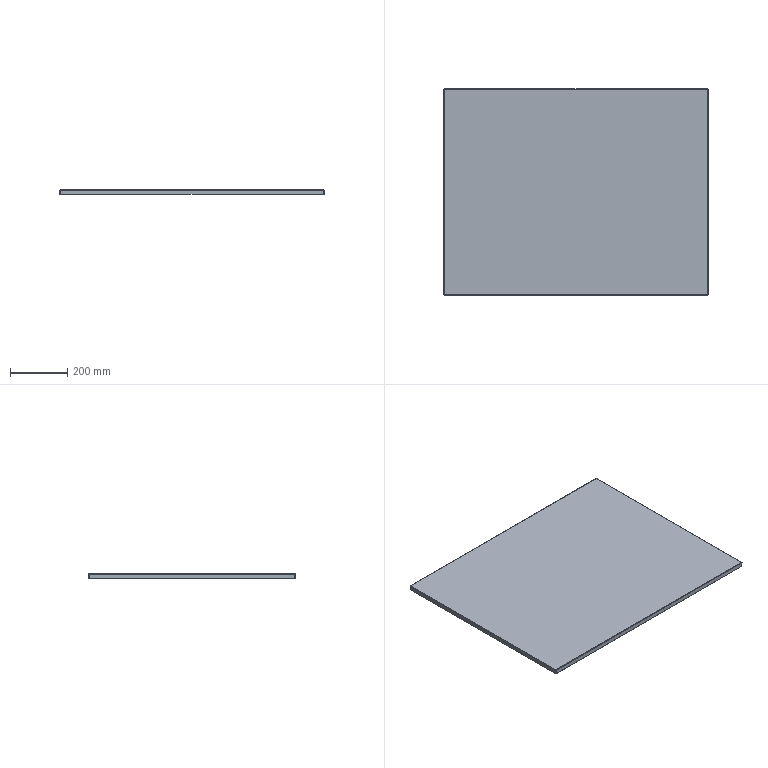Part | STEP file | Base plate | 1 solid | 38 faces | box 919 x 719 x 16.2 mm | volume 850250 mm3 | plane 22 | spline 8 | cylinder 8 | commonest cylinder face diameters 0.4 x4 2.8 x4
STEP:
#1=CARTESIAN_POINT('',(458.1,358.1,-1.2));
#2=VERTEX_POINT('',#1);
#3=CARTESIAN_POINT('',(-458.1,358.1,-1.2));
#4=VERTEX_POINT('',#3);
#5=CARTESIAN_POINT('',(458.1,358.1,-1.2));
#6=DIRECTION('',(-1.,0.,0.));
#7=VECTOR('',#6,1000.);
#8=LINE('',#5,#7);
#9=EDGE_CURVE('',#2,#4,#8,.T.);
#10=ORIENTED_EDGE('',*,*,#9,.F.);
#11=CARTESIAN_POINT('',(458.1,-358.1,-1.2));
#12=VERTEX_POINT('',#11);
#13=CARTESIAN_POINT('',(458.1,-358.1,-1.2));
#14=DIRECTION('',(0.,1.,0.));
#15=VECTOR('',#14,1000.);
#16=LINE('',#13,#15);
#17=EDGE_CURVE('',#12,#2,#16,.T.);
#18=ORIENTED_EDGE('',*,*,#17,.F.);
#19=CARTESIAN_POINT('',(-458.1,-358.1,-1.2));
#20=VERTEX_POINT('',#19);
#21=CARTESIAN_POINT('',(-458.1,-358.1,-1.2));
#22=DIRECTION('',(1.,0.,0.));
#23=VECTOR('',#22,1000.);
#24=LINE('',#21,#23);
#25=EDGE_CURVE('',#20,#12,#24,.T.);
#26=ORIENTED_EDGE('',*,*,#25,.F.);
#27=CARTESIAN_POINT('',(-458.1,358.1,-1.2));
#28=DIRECTION('',(0.,-1.,0.));
#29=VECTOR('',#28,1000.);
#30=LINE('',#27,#29);
#31=EDGE_CURVE('',#4,#20,#30,.T.);
#32=ORIENTED_EDGE('',*,*,#31,.F.);
#33=EDGE_LOOP('',(#10,#18,#26,#32));
#34=FACE_OUTER_BOUND('',#33,.T.);
#35=CARTESIAN_POINT('',(0.,0.,-1.2));
#36=DIRECTION('',(0.,0.,1.));
#37=DIRECTION('',(1.,0.,0.));
#38=AXIS2_PLACEMENT_3D('',#35,#36,#37);
#39=PLANE('',#38);
#40=ADVANCED_FACE('',(#34),#39,.F.);
#41=CARTESIAN_POINT('',(458.1,-358.1,0.));
#42=VERTEX_POINT('',#41);
#43=CARTESIAN_POINT('',(458.1,358.1,0.));
#44=VERTEX_POINT('',#43);
#45=CARTESIAN_POINT('',(458.1,-358.1,0.));
#46=DIRECTION('',(0.,1.,0.));
#47=VECTOR('',#46,1000.);
#48=LINE('',#45,#47);
#49=EDGE_CURVE('',#42,#44,#48,.T.);
#50=ORIENTED_EDGE('',*,*,#49,.T.);
#51=CARTESIAN_POINT('',(-458.1,358.1,0.));
#52=VERTEX_POINT('',#51);
#53=CARTESIAN_POINT('',(458.1,358.1,0.));
#54=DIRECTION('',(-1.,0.,0.));
#55=VECTOR('',#54,1000.);
#56=LINE('',#53,#55);
#57=EDGE_CURVE('',#44,#52,#56,.T.);
#58=ORIENTED_EDGE('',*,*,#57,.T.);
#59=CARTESIAN_POINT('',(-458.1,-358.1,0.));
#60=VERTEX_POINT('',#59);
#61=CARTESIAN_POINT('',(-458.1,358.1,0.));
#62=DIRECTION('',(0.,-1.,0.));
#63=VECTOR('',#62,1000.);
#64=LINE('',#61,#63);
#65=EDGE_CURVE('',#52,#60,#64,.T.);
#66=ORIENTED_EDGE('',*,*,#65,.T.);
#67=CARTESIAN_POINT('',(-458.1,-358.1,0.));
#68=DIRECTION('',(1.,0.,0.));
#69=VECTOR('',#68,1000.);
#70=LINE('',#67,#69);
#71=EDGE_CURVE('',#60,#42,#70,.T.);
#72=ORIENTED_EDGE('',*,*,#71,.T.);
#73=EDGE_LOOP('',(#50,#58,#66,#72));
#74=FACE_OUTER_BOUND('',#73,.T.);
#75=CARTESIAN_POINT('',(0.,0.,0.));
#76=DIRECTION('',(0.,0.,1.));
#77=DIRECTION('',(1.,0.,0.));
#78=AXIS2_PLACEMENT_3D('',#75,#76,#77);
#79=PLANE('',#78);
#80=ADVANCED_FACE('',(#74),#79,.T.);
#81=CARTESIAN_POINT('',(457.593,-359.5,-1.4));
#82=VERTEX_POINT('',#81);
#83=CARTESIAN_POINT('',(457.593,-358.3,-1.4));
#84=VERTEX_POINT('',#83);
#85=CARTESIAN_POINT('',(457.593,-358.3,-1.4));
#86=DIRECTION('',(0.,1.,0.));
#87=VECTOR('',#86,1000.);
#88=LINE('',#85,#87);
#89=EDGE_CURVE('',#82,#84,#88,.T.);
#90=ORIENTED_EDGE('',*,*,#89,.T.);
#91=CARTESIAN_POINT('',(458.1,-358.1,-1.2));
#92=CARTESIAN_POINT('',(458.015,-358.152,-1.2));
#93=CARTESIAN_POINT('',(457.931,-358.204,-1.222));
#94=CARTESIAN_POINT('',(457.762,-358.278,-1.296));
#95=CARTESIAN_POINT('',(457.677,-358.3,-1.348));
#96=CARTESIAN_POINT('',(457.593,-358.3,-1.4));
#97=B_SPLINE_CURVE_WITH_KNOTS('',3,(#91,#92,#93,#94,#95,#96),.UNSPECIFIED.,.F.,.F.,(4,2,4),(0.,0.5,1.),.UNSPECIFIED.);
#98=EDGE_CURVE('',#12,#84,#97,.T.);
#99=ORIENTED_EDGE('',*,*,#98,.F.);
#100=CARTESIAN_POINT('',(458.1,-358.1,-1.2));
#101=DIRECTION('',(0.,0.,1.));
#102=VECTOR('',#101,1000.);
#103=LINE('',#100,#102);
#104=EDGE_CURVE('',#12,#42,#103,.T.);
#105=ORIENTED_EDGE('',*,*,#104,.T.);
#106=CARTESIAN_POINT('',(458.1,-358.1,0.));
#107=CARTESIAN_POINT('',(458.058,-358.283,0.));
#108=CARTESIAN_POINT('',(458.015,-358.466,-0.03644));
#109=CARTESIAN_POINT('',(457.931,-358.805,-0.1767));
#110=CARTESIAN_POINT('',(457.889,-358.96,-0.2805));
#111=CARTESIAN_POINT('',(457.804,-359.22,-0.5396));
#112=CARTESIAN_POINT('',(457.762,-359.323,-0.6949));
#113=CARTESIAN_POINT('',(457.677,-359.464,-1.034));
#114=CARTESIAN_POINT('',(457.635,-359.5,-1.217));
#115=CARTESIAN_POINT('',(457.593,-359.5,-1.4));
#116=B_SPLINE_CURVE_WITH_KNOTS('',3,(#106,#107,#108,#109,#110,#111,#112,#113,#114,#115),.UNSPECIFIED.,.F.,.F.,(4,2,2,2,4),(0.,0.25,0.5,0.75,1.),.UNSPECIFIED.);
#117=EDGE_CURVE('',#42,#82,#116,.T.);
#118=ORIENTED_EDGE('',*,*,#117,.T.);
#119=EDGE_LOOP('',(#90,#99,#105,#118));
#120=FACE_OUTER_BOUND('',#119,.T.);
#121=CARTESIAN_POINT('',(458.1,-358.1,0.012));
#122=CARTESIAN_POINT('',(458.058,-358.285,0.012));
#123=CARTESIAN_POINT('',(458.015,-358.47,-0.02475));
#124=CARTESIAN_POINT('',(457.931,-358.811,-0.1662));
#125=CARTESIAN_POINT('',(457.889,-358.968,-0.2709));
#126=CARTESIAN_POINT('',(457.804,-359.229,-0.5323));
#127=CARTESIAN_POINT('',(457.762,-359.334,-0.6889));
#128=CARTESIAN_POINT('',(457.677,-359.475,-1.03));
#129=CARTESIAN_POINT('',(457.635,-359.512,-1.215));
#130=CARTESIAN_POINT('',(457.593,-359.512,-1.4));
#131=CARTESIAN_POINT('',(458.1,-358.1,0.));
#132=CARTESIAN_POINT('',(458.058,-358.283,0.));
#133=CARTESIAN_POINT('',(458.015,-358.466,-0.03644));
#134=CARTESIAN_POINT('',(457.931,-358.805,-0.1767));
#135=CARTESIAN_POINT('',(457.889,-358.96,-0.2805));
#136=CARTESIAN_POINT('',(457.804,-359.22,-0.5396));
#137=CARTESIAN_POINT('',(457.762,-359.323,-0.6949));
#138=CARTESIAN_POINT('',(457.677,-359.464,-1.034));
#139=CARTESIAN_POINT('',(457.635,-359.5,-1.217));
#140=CARTESIAN_POINT('',(457.593,-359.5,-1.4));
#141=CARTESIAN_POINT('',(458.1,-358.1,-1.2));
#142=CARTESIAN_POINT('',(458.058,-358.126,-1.2));
#143=CARTESIAN_POINT('',(458.015,-358.152,-1.205));
#144=CARTESIAN_POINT('',(457.931,-358.201,-1.225));
#145=CARTESIAN_POINT('',(457.889,-358.223,-1.24));
#146=CARTESIAN_POINT('',(457.804,-358.26,-1.277));
#147=CARTESIAN_POINT('',(457.762,-358.275,-1.299));
#148=CARTESIAN_POINT('',(457.677,-358.295,-1.348));
#149=CARTESIAN_POINT('',(457.635,-358.3,-1.374));
#150=CARTESIAN_POINT('',(457.593,-358.3,-1.4));
#151=CARTESIAN_POINT('',(458.1,-358.1,-1.212));
#152=CARTESIAN_POINT('',(458.058,-358.125,-1.212));
#153=CARTESIAN_POINT('',(458.015,-358.149,-1.217));
#154=CARTESIAN_POINT('',(457.931,-358.195,-1.236));
#155=CARTESIAN_POINT('',(457.889,-358.215,-1.25));
#156=CARTESIAN_POINT('',(457.804,-358.25,-1.285));
#157=CARTESIAN_POINT('',(457.762,-358.264,-1.305));
#158=CARTESIAN_POINT('',(457.677,-358.283,-1.351));
#159=CARTESIAN_POINT('',(457.635,-358.288,-1.375));
#160=CARTESIAN_POINT('',(457.593,-358.288,-1.4));
#161=B_SPLINE_SURFACE_WITH_KNOTS('',1,3,((#121,#122,#123,#124,#125,#126,#127,#128,#129,#130),(#131,#132,#133,#134,#135,#136,#137,#138,#139,#140),(#141,#142,#143,#144,#145,#146,#147,#148,#149,#150),(#151,#152,#153,#154,#155,#156,#157,#158,#159,#160)),.UNSPECIFIED.,.F.,.F.,.F.,(2,1,1,2),(4,2,2,2,4),(-0.01,0.,1.,1.01),(0.,0.25,0.5,0.75,1.),.UNSPECIFIED.);
#162=ADVANCED_FACE('',(#120),#161,.F.);
#163=CARTESIAN_POINT('',(-457.593,-358.3,-1.4));
#164=VERTEX_POINT('',#163);
#165=CARTESIAN_POINT('',(-457.593,-358.3,-1.4));
#166=CARTESIAN_POINT('',(-457.677,-358.3,-1.348));
#167=CARTESIAN_POINT('',(-457.762,-358.278,-1.296));
#168=CARTESIAN_POINT('',(-457.931,-358.204,-1.222));
#169=CARTESIAN_POINT('',(-458.015,-358.152,-1.2));
#170=CARTESIAN_POINT('',(-458.1,-358.1,-1.2));
#171=B_SPLINE_CURVE_WITH_KNOTS('',3,(#165,#166,#167,#168,#169,#170),.UNSPECIFIED.,.F.,.F.,(4,2,4),(0.,0.5,1.),.UNSPECIFIED.);
#172=EDGE_CURVE('',#164,#20,#171,.T.);
#173=ORIENTED_EDGE('',*,*,#172,.F.);
#174=CARTESIAN_POINT('',(-457.593,-359.5,-1.4));
#175=VERTEX_POINT('',#174);
#176=CARTESIAN_POINT('',(-457.593,-358.3,-1.4));
#177=DIRECTION('',(0.,1.,0.));
#178=VECTOR('',#177,1000.);
#179=LINE('',#176,#178);
#180=EDGE_CURVE('',#175,#164,#179,.T.);
#181=ORIENTED_EDGE('',*,*,#180,.F.);
#182=CARTESIAN_POINT('',(-457.593,-359.5,-1.4));
#183=CARTESIAN_POINT('',(-457.635,-359.5,-1.217));
#184=CARTESIAN_POINT('',(-457.677,-359.464,-1.034));
#185=CARTESIAN_POINT('',(-457.762,-359.323,-0.6949));
#186=CARTESIAN_POINT('',(-457.804,-359.22,-0.5396));
#187=CARTESIAN_POINT('',(-457.889,-358.96,-0.2805));
#188=CARTESIAN_POINT('',(-457.931,-358.805,-0.1767));
#189=CARTESIAN_POINT('',(-458.015,-358.466,-0.03644));
#190=CARTESIAN_POINT('',(-458.058,-358.283,0.));
#191=CARTESIAN_POINT('',(-458.1,-358.1,0.));
#192=B_SPLINE_CURVE_WITH_KNOTS('',3,(#182,#183,#184,#185,#186,#187,#188,#189,#190,#191),.UNSPECIFIED.,.F.,.F.,(4,2,2,2,4),(0.,0.25,0.5,0.75,1.),.UNSPECIFIED.);
#193=EDGE_CURVE('',#175,#60,#192,.T.);
#194=ORIENTED_EDGE('',*,*,#193,.T.);
#195=CARTESIAN_POINT('',(-458.1,-358.1,-1.2));
#196=DIRECTION('',(0.,0.,1.));
#197=VECTOR('',#196,1000.);
#198=LINE('',#195,#197);
#199=EDGE_CURVE('',#20,#60,#198,.T.);
#200=ORIENTED_EDGE('',*,*,#199,.F.);
#201=EDGE_LOOP('',(#173,#181,#194,#200));
#202=FACE_OUTER_BOUND('',#201,.T.);
#203=CARTESIAN_POINT('',(-457.593,-359.512,-1.4));
#204=CARTESIAN_POINT('',(-457.635,-359.512,-1.215));
#205=CARTESIAN_POINT('',(-457.677,-359.475,-1.03));
#206=CARTESIAN_POINT('',(-457.762,-359.334,-0.6889));
#207=CARTESIAN_POINT('',(-457.804,-359.229,-0.5323));
#208=CARTESIAN_POINT('',(-457.889,-358.968,-0.2709));
#209=CARTESIAN_POINT('',(-457.931,-358.811,-0.1662));
#210=CARTESIAN_POINT('',(-458.015,-358.47,-0.02475));
#211=CARTESIAN_POINT('',(-458.058,-358.285,0.012));
#212=CARTESIAN_POINT('',(-458.1,-358.1,0.012));
#213=CARTESIAN_POINT('',(-457.593,-359.5,-1.4));
#214=CARTESIAN_POINT('',(-457.635,-359.5,-1.217));
#215=CARTESIAN_POINT('',(-457.677,-359.464,-1.034));
#216=CARTESIAN_POINT('',(-457.762,-359.323,-0.6949));
#217=CARTESIAN_POINT('',(-457.804,-359.22,-0.5396));
#218=CARTESIAN_POINT('',(-457.889,-358.96,-0.2805));
#219=CARTESIAN_POINT('',(-457.931,-358.805,-0.1767));
#220=CARTESIAN_POINT('',(-458.015,-358.466,-0.03644));
#221=CARTESIAN_POINT('',(-458.058,-358.283,0.));
#222=CARTESIAN_POINT('',(-458.1,-358.1,0.));
#223=CARTESIAN_POINT('',(-457.593,-358.3,-1.4));
#224=CARTESIAN_POINT('',(-457.635,-358.3,-1.374));
#225=CARTESIAN_POINT('',(-457.677,-358.295,-1.348));
#226=CARTESIAN_POINT('',(-457.762,-358.275,-1.299));
#227=CARTESIAN_POINT('',(-457.804,-358.26,-1.277));
#228=CARTESIAN_POINT('',(-457.889,-358.223,-1.24));
#229=CARTESIAN_POINT('',(-457.931,-358.201,-1.225));
#230=CARTESIAN_POINT('',(-458.015,-358.152,-1.205));
#231=CARTESIAN_POINT('',(-458.058,-358.126,-1.2));
#232=CARTESIAN_POINT('',(-458.1,-358.1,-1.2));
#233=CARTESIAN_POINT('',(-457.593,-358.288,-1.4));
#234=CARTESIAN_POINT('',(-457.635,-358.288,-1.375));
#235=CARTESIAN_POINT('',(-457.677,-358.283,-1.351));
#236=CARTESIAN_POINT('',(-457.762,-358.264,-1.305));
#237=CARTESIAN_POINT('',(-457.804,-358.25,-1.285));
#238=CARTESIAN_POINT('',(-457.889,-358.215,-1.25));
#239=CARTESIAN_POINT('',(-457.931,-358.195,-1.236));
#240=CARTESIAN_POINT('',(-458.015,-358.149,-1.217));
#241=CARTESIAN_POINT('',(-458.058,-358.125,-1.212));
#242=CARTESIAN_POINT('',(-458.1,-358.1,-1.212));
#243=B_SPLINE_SURFACE_WITH_KNOTS('',1,3,((#203,#204,#205,#206,#207,#208,#209,#210,#211,#212),(#213,#214,#215,#216,#217,#218,#219,#220,#221,#222),(#223,#224,#225,#226,#227,#228,#229,#230,#231,#232),(#233,#234,#235,#236,#237,#238,#239,#240,#241,#242)),.UNSPECIFIED.,.F.,.F.,.F.,(2,1,1,2),(4,2,2,2,4),(-0.01,0.,1.,1.01),(0.,0.25,0.5,0.75,1.),.UNSPECIFIED.);
#244=ADVANCED_FACE('',(#202),#243,.F.);
#245=ORIENTED_EDGE('',*,*,#71,.F.);
#246=ORIENTED_EDGE('',*,*,#193,.F.);
#247=CARTESIAN_POINT('',(0.,-359.5,-1.4));
#248=DIRECTION('',(-1.,0.,0.));
#249=VECTOR('',#248,1000.);
#250=LINE('',#247,#249);
#251=EDGE_CURVE('',#82,#175,#250,.T.);
#252=ORIENTED_EDGE('',*,*,#251,.F.);
#253=ORIENTED_EDGE('',*,*,#117,.F.);
#254=EDGE_LOOP('',(#245,#246,#252,#253));
#255=FACE_OUTER_BOUND('',#254,.T.);
#256=CARTESIAN_POINT('',(-458.1,-358.1,-1.4));
#257=DIRECTION('',(-1.,0.,0.));
#258=DIRECTION('',(0.,-1.,0.));
#259=AXIS2_PLACEMENT_3D('',#256,#257,#258);
#260=CYLINDRICAL_SURFACE('',#259,1.4);
#261=ADVANCED_FACE('',(#255),#260,.T.);
#262=ORIENTED_EDGE('',*,*,#25,.T.);
#263=ORIENTED_EDGE('',*,*,#98,.T.);
#264=CARTESIAN_POINT('',(459.5,-358.3,-1.4));
#265=DIRECTION('',(-1.,0.,0.));
#266=VECTOR('',#265,1000.);
#267=LINE('',#264,#266);
#268=EDGE_CURVE('',#84,#164,#267,.T.);
#269=ORIENTED_EDGE('',*,*,#268,.T.);
#270=ORIENTED_EDGE('',*,*,#172,.T.);
#271=EDGE_LOOP('',(#262,#263,#269,#270));
#272=FACE_OUTER_BOUND('',#271,.T.);
#273=CARTESIAN_POINT('',(-458.1,-358.1,-1.4));
#274=DIRECTION('',(-1.,0.,0.));
#275=DIRECTION('',(0.,-1.,0.));
#276=AXIS2_PLACEMENT_3D('',#273,#274,#275);
#277=CYLINDRICAL_SURFACE('',#276,0.2);
#278=ADVANCED_FACE('',(#272),#277,.F.);
#279=CARTESIAN_POINT('',(457.593,-359.5,-16.2));
#280=VERTEX_POINT('',#279);
#281=CARTESIAN_POINT('',(457.593,-359.5,0.));
#282=DIRECTION('',(0.,0.,1.));
#283=VECTOR('',#282,1000.);
#284=LINE('',#281,#283);
#285=EDGE_CURVE('',#280,#82,#284,.T.);
#286=ORIENTED_EDGE('',*,*,#285,.F.);
#287=CARTESIAN_POINT('',(457.593,-358.3,-16.2));
#288=VERTEX_POINT('',#287);
#289=CARTESIAN_POINT('',(457.593,-358.3,-16.2));
#290=DIRECTION('',(0.,1.,0.));
#291=VECTOR('',#290,1000.);
#292=LINE('',#289,#291);
#293=EDGE_CURVE('',#280,#288,#292,.T.);
#294=ORIENTED_EDGE('',*,*,#293,.T.);
#295=CARTESIAN_POINT('',(457.593,-358.3,0.));
#296=DIRECTION('',(0.,0.,-1.));
#297=VECTOR('',#296,1000.);
#298=LINE('',#295,#297);
#299=EDGE_CURVE('',#84,#288,#298,.T.);
#300=ORIENTED_EDGE('',*,*,#299,.F.);
#301=ORIENTED_EDGE('',*,*,#89,.F.);
#302=EDGE_LOOP('',(#286,#294,#300,#301));
#303=FACE_OUTER_BOUND('',#302,.T.);
#304=CARTESIAN_POINT('',(457.593,-358.3,-1.2));
#305=DIRECTION('',(1.,0.,0.));
#306=DIRECTION('',(0.,0.,-1.));
#307=AXIS2_PLACEMENT_3D('',#304,#305,#306);
#308=PLANE('',#307);
#309=ADVANCED_FACE('',(#303),#308,.T.);
#310=CARTESIAN_POINT('',(-457.593,-359.5,-16.2));
#311=VERTEX_POINT('',#310);
#312=CARTESIAN_POINT('',(0.,-359.5,-16.2));
#313=DIRECTION('',(1.,0.,0.));
#314=VECTOR('',#313,1000.);
#315=LINE('',#312,#314);
#316=EDGE_CURVE('',#311,#280,#315,.T.);
#317=ORIENTED_EDGE('',*,*,#316,.T.);
#318=ORIENTED_EDGE('',*,*,#285,.T.);
#319=ORIENTED_EDGE('',*,*,#251,.T.);
#320=CARTESIAN_POINT('',(-457.593,-359.5,-1.2));
#321=DIRECTION('',(0.,0.,1.));
#322=VECTOR('',#321,1000.);
#323=LINE('',#320,#322);
#324=EDGE_CURVE('',#311,#175,#323,.T.);
#325=ORIENTED_EDGE('',*,*,#324,.F.);
#326=EDGE_LOOP('',(#317,#318,#319,#325));
#327=FACE_OUTER_BOUND('',#326,.T.);
#328=CARTESIAN_POINT('',(0.,-359.5,0.));
#329=DIRECTION('',(0.,-1.,0.));
#330=DIRECTION('',(0.,0.,-1.));
#331=AXIS2_PLACEMENT_3D('',#328,#329,#330);
#332=PLANE('',#331);
#333=ADVANCED_FACE('',(#327),#332,.T.);
#334=ORIENTED_EDGE('',*,*,#299,.T.);
#335=CARTESIAN_POINT('',(-457.593,-358.3,-16.2));
#336=VERTEX_POINT('',#335);
#337=CARTESIAN_POINT('',(-459.5,-358.3,-16.2));
#338=DIRECTION('',(1.,0.,0.));
#339=VECTOR('',#338,1000.);
#340=LINE('',#337,#339);
#341=EDGE_CURVE('',#336,#288,#340,.T.);
#342=ORIENTED_EDGE('',*,*,#341,.F.);
#343=CARTESIAN_POINT('',(-457.593,-358.3,-1.2));
#344=DIRECTION('',(0.,0.,-1.));
#345=VECTOR('',#344,1000.);
#346=LINE('',#343,#345);
#347=EDGE_CURVE('',#164,#336,#346,.T.);
#348=ORIENTED_EDGE('',*,*,#347,.F.);
#349=ORIENTED_EDGE('',*,*,#268,.F.);
#350=EDGE_LOOP('',(#334,#342,#348,#349));
#351=FACE_OUTER_BOUND('',#350,.T.);
#352=CARTESIAN_POINT('',(0.,-358.3,0.));
#353=DIRECTION('',(0.,-1.,0.));
#354=DIRECTION('',(0.,0.,-1.));
#355=AXIS2_PLACEMENT_3D('',#352,#353,#354);
#356=PLANE('',#355);
#357=ADVANCED_FACE('',(#351),#356,.F.);
#358=ORIENTED_EDGE('',*,*,#293,.F.);
#359=ORIENTED_EDGE('',*,*,#316,.F.);
#360=CARTESIAN_POINT('',(-457.593,-359.5,-16.2));
#361=DIRECTION('',(0.,1.,0.));
#362=VECTOR('',#361,1000.);
#363=LINE('',#360,#362);
#364=EDGE_CURVE('',#311,#336,#363,.T.);
#365=ORIENTED_EDGE('',*,*,#364,.T.);
#366=ORIENTED_EDGE('',*,*,#341,.T.);
#367=EDGE_LOOP('',(#358,#359,#365,#366));
#368=FACE_OUTER_BOUND('',#367,.T.);
#369=CARTESIAN_POINT('',(-459.5,-359.5,-16.2));
#370=DIRECTION('',(0.,0.,1.));
#371=DIRECTION('',(0.,-1.,0.));
#372=AXIS2_PLACEMENT_3D('',#369,#370,#371);
#373=PLANE('',#372);
#374=ADVANCED_FACE('',(#368),#373,.F.);
#375=ORIENTED_EDGE('',*,*,#364,.F.);
#376=ORIENTED_EDGE('',*,*,#324,.T.);
#377=ORIENTED_EDGE('',*,*,#180,.T.);
#378=ORIENTED_EDGE('',*,*,#347,.T.);
#379=EDGE_LOOP('',(#375,#376,#377,#378));
#380=FACE_OUTER_BOUND('',#379,.T.);
#381=CARTESIAN_POINT('',(-457.593,-358.3,-1.2));
#382=DIRECTION('',(1.,0.,0.));
#383=DIRECTION('',(0.,0.,-1.));
#384=AXIS2_PLACEMENT_3D('',#381,#382,#383);
#385=PLANE('',#384);
#386=ADVANCED_FACE('',(#380),#385,.F.);
#387=CARTESIAN_POINT('',(459.5,357.593,-1.4));
#388=VERTEX_POINT('',#387);
#389=CARTESIAN_POINT('',(458.3,357.593,-1.4));
#390=VERTEX_POINT('',#389);
#391=CARTESIAN_POINT('',(458.3,357.593,-1.4));
#392=DIRECTION('',(-1.,0.,0.));
#393=VECTOR('',#392,1000.);
#394=LINE('',#391,#393);
#395=EDGE_CURVE('',#388,#390,#394,.T.);
#396=ORIENTED_EDGE('',*,*,#395,.T.);
#397=CARTESIAN_POINT('',(458.1,358.1,-1.2));
#398=CARTESIAN_POINT('',(458.152,358.015,-1.2));
#399=CARTESIAN_POINT('',(458.204,357.931,-1.222));
#400=CARTESIAN_POINT('',(458.278,357.762,-1.296));
#401=CARTESIAN_POINT('',(458.3,357.677,-1.348));
#402=CARTESIAN_POINT('',(458.3,357.593,-1.4));
#403=B_SPLINE_CURVE_WITH_KNOTS('',3,(#397,#398,#399,#400,#401,#402),.UNSPECIFIED.,.F.,.F.,(4,2,4),(0.,0.5,1.),.UNSPECIFIED.);
#404=EDGE_CURVE('',#2,#390,#403,.T.);
#405=ORIENTED_EDGE('',*,*,#404,.F.);
#406=CARTESIAN_POINT('',(458.1,358.1,-1.2));
#407=DIRECTION('',(0.,0.,1.));
#408=VECTOR('',#407,1000.);
#409=LINE('',#406,#408);
#410=EDGE_CURVE('',#2,#44,#409,.T.);
#411=ORIENTED_EDGE('',*,*,#410,.T.);
#412=CARTESIAN_POINT('',(458.1,358.1,0.));
#413=CARTESIAN_POINT('',(458.283,358.058,0.));
#414=CARTESIAN_POINT('',(458.466,358.015,-0.03644));
#415=CARTESIAN_POINT('',(458.805,357.931,-0.1767));
#416=CARTESIAN_POINT('',(458.96,357.889,-0.2805));
#417=CARTESIAN_POINT('',(459.22,357.804,-0.5396));
#418=CARTESIAN_POINT('',(459.323,357.762,-0.6949));
#419=CARTESIAN_POINT('',(459.464,357.677,-1.034));
#420=CARTESIAN_POINT('',(459.5,357.635,-1.217));
#421=CARTESIAN_POINT('',(459.5,357.593,-1.4));
#422=B_SPLINE_CURVE_WITH_KNOTS('',3,(#412,#413,#414,#415,#416,#417,#418,#419,#420,#421),.UNSPECIFIED.,.F.,.F.,(4,2,2,2,4),(0.,0.25,0.5,0.75,1.),.UNSPECIFIED.);
#423=EDGE_CURVE('',#44,#388,#422,.T.);
#424=ORIENTED_EDGE('',*,*,#423,.T.);
#425=EDGE_LOOP('',(#396,#405,#411,#424));
#426=FACE_OUTER_BOUND('',#425,.T.);
#427=CARTESIAN_POINT('',(458.1,358.1,0.012));
#428=CARTESIAN_POINT('',(458.285,358.058,0.012));
#429=CARTESIAN_POINT('',(458.47,358.015,-0.02475));
#430=CARTESIAN_POINT('',(458.811,357.931,-0.1662));
#431=CARTESIAN_POINT('',(458.968,357.889,-0.2709));
#432=CARTESIAN_POINT('',(459.229,357.804,-0.5323));
#433=CARTESIAN_POINT('',(459.334,357.762,-0.6889));
#434=CARTESIAN_POINT('',(459.475,357.677,-1.03));
#435=CARTESIAN_POINT('',(459.512,357.635,-1.215));
#436=CARTESIAN_POINT('',(459.512,357.593,-1.4));
#437=CARTESIAN_POINT('',(458.1,358.1,0.));
#438=CARTESIAN_POINT('',(458.283,358.058,0.));
#439=CARTESIAN_POINT('',(458.466,358.015,-0.03644));
#440=CARTESIAN_POINT('',(458.805,357.931,-0.1767));
#441=CARTESIAN_POINT('',(458.96,357.889,-0.2805));
#442=CARTESIAN_POINT('',(459.22,357.804,-0.5396));
#443=CARTESIAN_POINT('',(459.323,357.762,-0.6949));
#444=CARTESIAN_POINT('',(459.464,357.677,-1.034));
#445=CARTESIAN_POINT('',(459.5,357.635,-1.217));
#446=CARTESIAN_POINT('',(459.5,357.593,-1.4));
#447=CARTESIAN_POINT('',(458.1,358.1,-1.2));
#448=CARTESIAN_POINT('',(458.126,358.058,-1.2));
#449=CARTESIAN_POINT('',(458.152,358.015,-1.205));
#450=CARTESIAN_POINT('',(458.201,357.931,-1.225));
#451=CARTESIAN_POINT('',(458.223,357.889,-1.24));
#452=CARTESIAN_POINT('',(458.26,357.804,-1.277));
#453=CARTESIAN_POINT('',(458.275,357.762,-1.299));
#454=CARTESIAN_POINT('',(458.295,357.677,-1.348));
#455=CARTESIAN_POINT('',(458.3,357.635,-1.374));
#456=CARTESIAN_POINT('',(458.3,357.593,-1.4));
#457=CARTESIAN_POINT('',(458.1,358.1,-1.212));
#458=CARTESIAN_POINT('',(458.125,358.058,-1.212));
#459=CARTESIAN_POINT('',(458.149,358.015,-1.217));
#460=CARTESIAN_POINT('',(458.195,357.931,-1.236));
#461=CARTESIAN_POINT('',(458.215,357.889,-1.25));
#462=CARTESIAN_POINT('',(458.25,357.804,-1.285));
#463=CARTESIAN_POINT('',(458.264,357.762,-1.305));
#464=CARTESIAN_POINT('',(458.283,357.677,-1.351));
#465=CARTESIAN_POINT('',(458.288,357.635,-1.375));
#466=CARTESIAN_POINT('',(458.288,357.593,-1.4));
#467=B_SPLINE_SURFACE_WITH_KNOTS('',1,3,((#427,#428,#429,#430,#431,#432,#433,#434,#435,#436),(#437,#438,#439,#440,#441,#442,#443,#444,#445,#446),(#447,#448,#449,#450,#451,#452,#453,#454,#455,#456),(#457,#458,#459,#460,#461,#462,#463,#464,#465,#466)),.UNSPECIFIED.,.F.,.F.,.F.,(2,1,1,2),(4,2,2,2,4),(-0.01,0.,1.,1.01),(0.,0.25,0.5,0.75,1.),.UNSPECIFIED.);
#468=ADVANCED_FACE('',(#426),#467,.F.);
#469=CARTESIAN_POINT('',(458.3,-357.593,-1.4));
#470=VERTEX_POINT('',#469);
#471=CARTESIAN_POINT('',(458.3,-357.593,-1.4));
#472=CARTESIAN_POINT('',(458.3,-357.677,-1.348));
#473=CARTESIAN_POINT('',(458.278,-357.762,-1.296));
#474=CARTESIAN_POINT('',(458.204,-357.931,-1.222));
#475=CARTESIAN_POINT('',(458.152,-358.015,-1.2));
#476=CARTESIAN_POINT('',(458.1,-358.1,-1.2));
#477=B_SPLINE_CURVE_WITH_KNOTS('',3,(#471,#472,#473,#474,#475,#476),.UNSPECIFIED.,.F.,.F.,(4,2,4),(0.,0.5,1.),.UNSPECIFIED.);
#478=EDGE_CURVE('',#470,#12,#477,.T.);
#479=ORIENTED_EDGE('',*,*,#478,.F.);
#480=CARTESIAN_POINT('',(459.5,-357.593,-1.4));
#481=VERTEX_POINT('',#480);
#482=CARTESIAN_POINT('',(458.3,-357.593,-1.4));
#483=DIRECTION('',(-1.,0.,0.));
#484=VECTOR('',#483,1000.);
#485=LINE('',#482,#484);
#486=EDGE_CURVE('',#481,#470,#485,.T.);
#487=ORIENTED_EDGE('',*,*,#486,.F.);
#488=CARTESIAN_POINT('',(459.5,-357.593,-1.4));
#489=CARTESIAN_POINT('',(459.5,-357.635,-1.217));
#490=CARTESIAN_POINT('',(459.464,-357.677,-1.034));
#491=CARTESIAN_POINT('',(459.323,-357.762,-0.6949));
#492=CARTESIAN_POINT('',(459.22,-357.804,-0.5396));
#493=CARTESIAN_POINT('',(458.96,-357.889,-0.2805));
#494=CARTESIAN_POINT('',(458.805,-357.931,-0.1767));
#495=CARTESIAN_POINT('',(458.466,-358.015,-0.03644));
#496=CARTESIAN_POINT('',(458.283,-358.058,0.));
#497=CARTESIAN_POINT('',(458.1,-358.1,0.));
#498=B_SPLINE_CURVE_WITH_KNOTS('',3,(#488,#489,#490,#491,#492,#493,#494,#495,#496,#497),.UNSPECIFIED.,.F.,.F.,(4,2,2,2,4),(0.,0.25,0.5,0.75,1.),.UNSPECIFIED.);
#499=EDGE_CURVE('',#481,#42,#498,.T.);
#500=ORIENTED_EDGE('',*,*,#499,.T.);
#501=ORIENTED_EDGE('',*,*,#104,.F.);
#502=EDGE_LOOP('',(#479,#487,#500,#501));
#503=FACE_OUTER_BOUND('',#502,.T.);
#504=CARTESIAN_POINT('',(459.512,-357.593,-1.4));
#505=CARTESIAN_POINT('',(459.512,-357.635,-1.215));
#506=CARTESIAN_POINT('',(459.475,-357.677,-1.03));
#507=CARTESIAN_POINT('',(459.334,-357.762,-0.6889));
#508=CARTESIAN_POINT('',(459.229,-357.804,-0.5323));
#509=CARTESIAN_POINT('',(458.968,-357.889,-0.2709));
#510=CARTESIAN_POINT('',(458.811,-357.931,-0.1662));
#511=CARTESIAN_POINT('',(458.47,-358.015,-0.02475));
#512=CARTESIAN_POINT('',(458.285,-358.058,0.012));
#513=CARTESIAN_POINT('',(458.1,-358.1,0.012));
#514=CARTESIAN_POINT('',(459.5,-357.593,-1.4));
#515=CARTESIAN_POINT('',(459.5,-357.635,-1.217));
#516=CARTESIAN_POINT('',(459.464,-357.677,-1.034));
#517=CARTESIAN_POINT('',(459.323,-357.762,-0.6949));
#518=CARTESIAN_POINT('',(459.22,-357.804,-0.5396));
#519=CARTESIAN_POINT('',(458.96,-357.889,-0.2805));
#520=CARTESIAN_POINT('',(458.805,-357.931,-0.1767));
#521=CARTESIAN_POINT('',(458.466,-358.015,-0.03644));
#522=CARTESIAN_POINT('',(458.283,-358.058,0.));
#523=CARTESIAN_POINT('',(458.1,-358.1,0.));
#524=CARTESIAN_POINT('',(458.3,-357.593,-1.4));
#525=CARTESIAN_POINT('',(458.3,-357.635,-1.374));
#526=CARTESIAN_POINT('',(458.295,-357.677,-1.348));
#527=CARTESIAN_POINT('',(458.275,-357.762,-1.299));
#528=CARTESIAN_POINT('',(458.26,-357.804,-1.277));
#529=CARTESIAN_POINT('',(458.223,-357.889,-1.24));
#530=CARTESIAN_POINT('',(458.201,-357.931,-1.225));
#531=CARTESIAN_POINT('',(458.152,-358.015,-1.205));
#532=CARTESIAN_POINT('',(458.126,-358.058,-1.2));
#533=CARTESIAN_POINT('',(458.1,-358.1,-1.2));
#534=CARTESIAN_POINT('',(458.288,-357.593,-1.4));
#535=CARTESIAN_POINT('',(458.288,-357.635,-1.375));
#536=CARTESIAN_POINT('',(458.283,-357.677,-1.351));
#537=CARTESIAN_POINT('',(458.264,-357.762,-1.305));
#538=CARTESIAN_POINT('',(458.25,-357.804,-1.285));
#539=CARTESIAN_POINT('',(458.215,-357.889,-1.25));
#540=CARTESIAN_POINT('',(458.195,-357.931,-1.236));
#541=CARTESIAN_POINT('',(458.149,-358.015,-1.217));
#542=CARTESIAN_POINT('',(458.125,-358.058,-1.212));
#543=CARTESIAN_POINT('',(458.1,-358.1,-1.212));
#544=B_SPLINE_SURFACE_WITH_KNOTS('',1,3,((#504,#505,#506,#507,#508,#509,#510,#511,#512,#513),(#514,#515,#516,#517,#518,#519,#520,#521,#522,#523),(#524,#525,#526,#527,#528,#529,#530,#531,#532,#533),(#534,#535,#536,#537,#538,#539,#540,#541,#542,#543)),.UNSPECIFIED.,.F.,.F.,.F.,(2,1,1,2),(4,2,2,2,4),(-0.01,0.,1.,1.01),(0.,0.25,0.5,0.75,1.),.UNSPECIFIED.);
#545=ADVANCED_FACE('',(#503),#544,.F.);
#546=ORIENTED_EDGE('',*,*,#49,.F.);
#547=ORIENTED_EDGE('',*,*,#499,.F.);
#548=CARTESIAN_POINT('',(459.5,0.,-1.4));
#549=DIRECTION('',(0.,-1.,0.));
#550=VECTOR('',#549,1000.);
#551=LINE('',#548,#550);
#552=EDGE_CURVE('',#388,#481,#551,.T.);
#553=ORIENTED_EDGE('',*,*,#552,.F.);
#554=ORIENTED_EDGE('',*,*,#423,.F.);
#555=EDGE_LOOP('',(#546,#547,#553,#554));
#556=FACE_OUTER_BOUND('',#555,.T.);
#557=CARTESIAN_POINT('',(458.1,-358.1,-1.4));
#558=DIRECTION('',(0.,-1.,0.));
#559=DIRECTION('',(1.,0.,0.));
#560=AXIS2_PLACEMENT_3D('',#557,#558,#559);
#561=CYLINDRICAL_SURFACE('',#560,1.4);
#562=ADVANCED_FACE('',(#556),#561,.T.);
#563=ORIENTED_EDGE('',*,*,#17,.T.);
#564=ORIENTED_EDGE('',*,*,#404,.T.);
#565=CARTESIAN_POINT('',(458.3,359.5,-1.4));
#566=DIRECTION('',(0.,-1.,0.));
#567=VECTOR('',#566,1000.);
#568=LINE('',#565,#567);
#569=EDGE_CURVE('',#390,#470,#568,.T.);
#570=ORIENTED_EDGE('',*,*,#569,.T.);
#571=ORIENTED_EDGE('',*,*,#478,.T.);
#572=EDGE_LOOP('',(#563,#564,#570,#571));
#573=FACE_OUTER_BOUND('',#572,.T.);
#574=CARTESIAN_POINT('',(458.1,-358.1,-1.4));
#575=DIRECTION('',(0.,-1.,0.));
#576=DIRECTION('',(1.,0.,0.));
#577=AXIS2_PLACEMENT_3D('',#574,#575,#576);
#578=CYLINDRICAL_SURFACE('',#577,0.2);
#579=ADVANCED_FACE('',(#573),#578,.F.);
#580=CARTESIAN_POINT('',(459.5,357.593,-16.2));
#581=VERTEX_POINT('',#580);
#582=CARTESIAN_POINT('',(459.5,357.593,0.));
#583=DIRECTION('',(0.,0.,1.));
#584=VECTOR('',#583,1000.);
#585=LINE('',#582,#584);
#586=EDGE_CURVE('',#581,#388,#585,.T.);
#587=ORIENTED_EDGE('',*,*,#586,.F.);
#588=CARTESIAN_POINT('',(458.3,357.593,-16.2));
#589=VERTEX_POINT('',#588);
#590=CARTESIAN_POINT('',(458.3,357.593,-16.2));
#591=DIRECTION('',(-1.,0.,0.));
#592=VECTOR('',#591,1000.);
#593=LINE('',#590,#592);
#594=EDGE_CURVE('',#581,#589,#593,.T.);
#595=ORIENTED_EDGE('',*,*,#594,.T.);
#596=CARTESIAN_POINT('',(458.3,357.593,0.));
#597=DIRECTION('',(0.,0.,-1.));
#598=VECTOR('',#597,1000.);
#599=LINE('',#596,#598);
#600=EDGE_CURVE('',#390,#589,#599,.T.);
#601=ORIENTED_EDGE('',*,*,#600,.F.);
#602=ORIENTED_EDGE('',*,*,#395,.F.);
#603=EDGE_LOOP('',(#587,#595,#601,#602));
#604=FACE_OUTER_BOUND('',#603,.T.);
#605=CARTESIAN_POINT('',(458.3,357.593,-1.2));
#606=DIRECTION('',(0.,1.,0.));
#607=DIRECTION('',(0.,0.,1.));
#608=AXIS2_PLACEMENT_3D('',#605,#606,#607);
#609=PLANE('',#608);
#610=ADVANCED_FACE('',(#604),#609,.T.);
#611=CARTESIAN_POINT('',(459.5,-357.593,-16.2));
#612=VERTEX_POINT('',#611);
#613=CARTESIAN_POINT('',(459.5,0.,-16.2));
#614=DIRECTION('',(0.,1.,0.));
#615=VECTOR('',#614,1000.);
#616=LINE('',#613,#615);
#617=EDGE_CURVE('',#612,#581,#616,.T.);
#618=ORIENTED_EDGE('',*,*,#617,.T.);
#619=ORIENTED_EDGE('',*,*,#586,.T.);
#620=ORIENTED_EDGE('',*,*,#552,.T.);
#621=CARTESIAN_POINT('',(459.5,-357.593,-1.2));
#622=DIRECTION('',(0.,0.,1.));
#623=VECTOR('',#622,1000.);
#624=LINE('',#621,#623);
#625=EDGE_CURVE('',#612,#481,#624,.T.);
#626=ORIENTED_EDGE('',*,*,#625,.F.);
#627=EDGE_LOOP('',(#618,#619,#620,#626));
#628=FACE_OUTER_BOUND('',#627,.T.);
#629=CARTESIAN_POINT('',(459.5,0.,0.));
#630=DIRECTION('',(1.,0.,0.));
#631=DIRECTION('',(0.,0.,-1.));
#632=AXIS2_PLACEMENT_3D('',#629,#630,#631);
#633=PLANE('',#632);
#634=ADVANCED_FACE('',(#628),#633,.T.);
#635=ORIENTED_EDGE('',*,*,#600,.T.);
#636=CARTESIAN_POINT('',(458.3,-357.593,-16.2));
#637=VERTEX_POINT('',#636);
#638=CARTESIAN_POINT('',(458.3,-359.5,-16.2));
#639=DIRECTION('',(0.,1.,0.));
#640=VECTOR('',#639,1000.);
#641=LINE('',#638,#640);
#642=EDGE_CURVE('',#637,#589,#641,.T.);
#643=ORIENTED_EDGE('',*,*,#642,.F.);
#644=CARTESIAN_POINT('',(458.3,-357.593,-1.2));
#645=DIRECTION('',(0.,0.,-1.));
#646=VECTOR('',#645,1000.);
#647=LINE('',#644,#646);
#648=EDGE_CURVE('',#470,#637,#647,.T.);
#649=ORIENTED_EDGE('',*,*,#648,.F.);
#650=ORIENTED_EDGE('',*,*,#569,.F.);
#651=EDGE_LOOP('',(#635,#643,#649,#650));
#652=FACE_OUTER_BOUND('',#651,.T.);
#653=CARTESIAN_POINT('',(458.3,0.,0.));
#654=DIRECTION('',(1.,0.,0.));
#655=DIRECTION('',(0.,0.,-1.));
#656=AXIS2_PLACEMENT_3D('',#653,#654,#655);
#657=PLANE('',#656);
#658=ADVANCED_FACE('',(#652),#657,.F.);
#659=ORIENTED_EDGE('',*,*,#594,.F.);
#660=ORIENTED_EDGE('',*,*,#617,.F.);
#661=CARTESIAN_POINT('',(459.5,-357.593,-16.2));
#662=DIRECTION('',(-1.,0.,0.));
#663=VECTOR('',#662,1000.);
#664=LINE('',#661,#663);
#665=EDGE_CURVE('',#612,#637,#664,.T.);
#666=ORIENTED_EDGE('',*,*,#665,.T.);
#667=ORIENTED_EDGE('',*,*,#642,.T.);
#668=EDGE_LOOP('',(#659,#660,#666,#667));
#669=FACE_OUTER_BOUND('',#668,.T.);
#670=CARTESIAN_POINT('',(459.5,-359.5,-16.2));
#671=DIRECTION('',(0.,0.,1.));
#672=DIRECTION('',(1.,0.,0.));
#673=AXIS2_PLACEMENT_3D('',#670,#671,#672);
#674=PLANE('',#673);
#675=ADVANCED_FACE('',(#669),#674,.F.);
#676=ORIENTED_EDGE('',*,*,#665,.F.);
#677=ORIENTED_EDGE('',*,*,#625,.T.);
#678=ORIENTED_EDGE('',*,*,#486,.T.);
#679=ORIENTED_EDGE('',*,*,#648,.T.);
#680=EDGE_LOOP('',(#676,#677,#678,#679));
#681=FACE_OUTER_BOUND('',#680,.T.);
#682=CARTESIAN_POINT('',(458.3,-357.593,-1.2));
#683=DIRECTION('',(0.,1.,0.));
#684=DIRECTION('',(0.,0.,1.));
#685=AXIS2_PLACEMENT_3D('',#682,#683,#684);
#686=PLANE('',#685);
#687=ADVANCED_FACE('',(#681),#686,.F.);
#688=CARTESIAN_POINT('',(-459.5,-357.593,-1.4));
#689=VERTEX_POINT('',#688);
#690=CARTESIAN_POINT('',(-458.3,-357.593,-1.4));
#691=VERTEX_POINT('',#690);
#692=CARTESIAN_POINT('',(-458.3,-357.593,-1.4));
#693=DIRECTION('',(1.,0.,0.));
#694=VECTOR('',#693,1000.);
#695=LINE('',#692,#694);
#696=EDGE_CURVE('',#689,#691,#695,.T.);
#697=ORIENTED_EDGE('',*,*,#696,.T.);
#698=CARTESIAN_POINT('',(-458.1,-358.1,-1.2));
#699=CARTESIAN_POINT('',(-458.152,-358.015,-1.2));
#700=CARTESIAN_POINT('',(-458.204,-357.931,-1.222));
#701=CARTESIAN_POINT('',(-458.278,-357.762,-1.296));
#702=CARTESIAN_POINT('',(-458.3,-357.677,-1.348));
#703=CARTESIAN_POINT('',(-458.3,-357.593,-1.4));
#704=B_SPLINE_CURVE_WITH_KNOTS('',3,(#698,#699,#700,#701,#702,#703),.UNSPECIFIED.,.F.,.F.,(4,2,4),(0.,0.5,1.),.UNSPECIFIED.);
#705=EDGE_CURVE('',#20,#691,#704,.T.);
#706=ORIENTED_EDGE('',*,*,#705,.F.);
#707=ORIENTED_EDGE('',*,*,#199,.T.);
#708=CARTESIAN_POINT('',(-458.1,-358.1,0.));
#709=CARTESIAN_POINT('',(-458.283,-358.058,0.));
#710=CARTESIAN_POINT('',(-458.466,-358.015,-0.03644));
#711=CARTESIAN_POINT('',(-458.805,-357.931,-0.1767));
#712=CARTESIAN_POINT('',(-458.96,-357.889,-0.2805));
#713=CARTESIAN_POINT('',(-459.22,-357.804,-0.5396));
#714=CARTESIAN_POINT('',(-459.323,-357.762,-0.6949));
#715=CARTESIAN_POINT('',(-459.464,-357.677,-1.034));
#716=CARTESIAN_POINT('',(-459.5,-357.635,-1.217));
#717=CARTESIAN_POINT('',(-459.5,-357.593,-1.4));
#718=B_SPLINE_CURVE_WITH_KNOTS('',3,(#708,#709,#710,#711,#712,#713,#714,#715,#716,#717),.UNSPECIFIED.,.F.,.F.,(4,2,2,2,4),(0.,0.25,0.5,0.75,1.),.UNSPECIFIED.);
#719=EDGE_CURVE('',#60,#689,#718,.T.);
#720=ORIENTED_EDGE('',*,*,#719,.T.);
#721=EDGE_LOOP('',(#697,#706,#707,#720));
#722=FACE_OUTER_BOUND('',#721,.T.);
#723=CARTESIAN_POINT('',(-458.1,-358.1,0.012));
#724=CARTESIAN_POINT('',(-458.285,-358.058,0.012));
#725=CARTESIAN_POINT('',(-458.47,-358.015,-0.02475));
#726=CARTESIAN_POINT('',(-458.811,-357.931,-0.1662));
#727=CARTESIAN_POINT('',(-458.968,-357.889,-0.2709));
#728=CARTESIAN_POINT('',(-459.229,-357.804,-0.5323));
#729=CARTESIAN_POINT('',(-459.334,-357.762,-0.6889));
#730=CARTESIAN_POINT('',(-459.475,-357.677,-1.03));
#731=CARTESIAN_POINT('',(-459.512,-357.635,-1.215));
#732=CARTESIAN_POINT('',(-459.512,-357.593,-1.4));
#733=CARTESIAN_POINT('',(-458.1,-358.1,0.));
#734=CARTESIAN_POINT('',(-458.283,-358.058,0.));
#735=CARTESIAN_POINT('',(-458.466,-358.015,-0.03644));
#736=CARTESIAN_POINT('',(-458.805,-357.931,-0.1767));
#737=CARTESIAN_POINT('',(-458.96,-357.889,-0.2805));
#738=CARTESIAN_POINT('',(-459.22,-357.804,-0.5396));
#739=CARTESIAN_POINT('',(-459.323,-357.762,-0.6949));
#740=CARTESIAN_POINT('',(-459.464,-357.677,-1.034));
#741=CARTESIAN_POINT('',(-459.5,-357.635,-1.217));
#742=CARTESIAN_POINT('',(-459.5,-357.593,-1.4));
#743=CARTESIAN_POINT('',(-458.1,-358.1,-1.2));
#744=CARTESIAN_POINT('',(-458.126,-358.058,-1.2));
#745=CARTESIAN_POINT('',(-458.152,-358.015,-1.205));
#746=CARTESIAN_POINT('',(-458.201,-357.931,-1.225));
#747=CARTESIAN_POINT('',(-458.223,-357.889,-1.24));
#748=CARTESIAN_POINT('',(-458.26,-357.804,-1.277));
#749=CARTESIAN_POINT('',(-458.275,-357.762,-1.299));
#750=CARTESIAN_POINT('',(-458.295,-357.677,-1.348));
#751=CARTESIAN_POINT('',(-458.3,-357.635,-1.374));
#752=CARTESIAN_POINT('',(-458.3,-357.593,-1.4));
#753=CARTESIAN_POINT('',(-458.1,-358.1,-1.212));
#754=CARTESIAN_POINT('',(-458.125,-358.058,-1.212));
#755=CARTESIAN_POINT('',(-458.149,-358.015,-1.217));
#756=CARTESIAN_POINT('',(-458.195,-357.931,-1.236));
#757=CARTESIAN_POINT('',(-458.215,-357.889,-1.25));
#758=CARTESIAN_POINT('',(-458.25,-357.804,-1.285));
#759=CARTESIAN_POINT('',(-458.264,-357.762,-1.305));
#760=CARTESIAN_POINT('',(-458.283,-357.677,-1.351));
#761=CARTESIAN_POINT('',(-458.288,-357.635,-1.375));
#762=CARTESIAN_POINT('',(-458.288,-357.593,-1.4));
#763=B_SPLINE_SURFACE_WITH_KNOTS('',1,3,((#723,#724,#725,#726,#727,#728,#729,#730,#731,#732),(#733,#734,#735,#736,#737,#738,#739,#740,#741,#742),(#743,#744,#745,#746,#747,#748,#749,#750,#751,#752),(#753,#754,#755,#756,#757,#758,#759,#760,#761,#762)),.UNSPECIFIED.,.F.,.F.,.F.,(2,1,1,2),(4,2,2,2,4),(-0.01,0.,1.,1.01),(0.,0.25,0.5,0.75,1.),.UNSPECIFIED.);
#764=ADVANCED_FACE('',(#722),#763,.F.);
#765=CARTESIAN_POINT('',(-458.3,357.593,-1.4));
#766=VERTEX_POINT('',#765);
#767=CARTESIAN_POINT('',(-458.3,357.593,-1.4));
#768=CARTESIAN_POINT('',(-458.3,357.677,-1.348));
#769=CARTESIAN_POINT('',(-458.278,357.762,-1.296));
#770=CARTESIAN_POINT('',(-458.204,357.931,-1.222));
#771=CARTESIAN_POINT('',(-458.152,358.015,-1.2));
#772=CARTESIAN_POINT('',(-458.1,358.1,-1.2));
#773=B_SPLINE_CURVE_WITH_KNOTS('',3,(#767,#768,#769,#770,#771,#772),.UNSPECIFIED.,.F.,.F.,(4,2,4),(0.,0.5,1.),.UNSPECIFIED.);
#774=EDGE_CURVE('',#766,#4,#773,.T.);
#775=ORIENTED_EDGE('',*,*,#774,.F.);
#776=CARTESIAN_POINT('',(-459.5,357.593,-1.4));
#777=VERTEX_POINT('',#776);
#778=CARTESIAN_POINT('',(-458.3,357.593,-1.4));
#779=DIRECTION('',(1.,0.,0.));
#780=VECTOR('',#779,1000.);
#781=LINE('',#778,#780);
#782=EDGE_CURVE('',#777,#766,#781,.T.);
#783=ORIENTED_EDGE('',*,*,#782,.F.);
#784=CARTESIAN_POINT('',(-459.5,357.593,-1.4));
#785=CARTESIAN_POINT('',(-459.5,357.635,-1.217));
#786=CARTESIAN_POINT('',(-459.464,357.677,-1.034));
#787=CARTESIAN_POINT('',(-459.323,357.762,-0.6949));
#788=CARTESIAN_POINT('',(-459.22,357.804,-0.5396));
#789=CARTESIAN_POINT('',(-458.96,357.889,-0.2805));
#790=CARTESIAN_POINT('',(-458.805,357.931,-0.1767));
#791=CARTESIAN_POINT('',(-458.466,358.015,-0.03644));
#792=CARTESIAN_POINT('',(-458.283,358.058,0.));
#793=CARTESIAN_POINT('',(-458.1,358.1,0.));
#794=B_SPLINE_CURVE_WITH_KNOTS('',3,(#784,#785,#786,#787,#788,#789,#790,#791,#792,#793),.UNSPECIFIED.,.F.,.F.,(4,2,2,2,4),(0.,0.25,0.5,0.75,1.),.UNSPECIFIED.);
#795=EDGE_CURVE('',#777,#52,#794,.T.);
#796=ORIENTED_EDGE('',*,*,#795,.T.);
#797=CARTESIAN_POINT('',(-458.1,358.1,-1.2));
#798=DIRECTION('',(0.,0.,1.));
#799=VECTOR('',#798,1000.);
#800=LINE('',#797,#799);
#801=EDGE_CURVE('',#4,#52,#800,.T.);
#802=ORIENTED_EDGE('',*,*,#801,.F.);
#803=EDGE_LOOP('',(#775,#783,#796,#802));
#804=FACE_OUTER_BOUND('',#803,.T.);
#805=CARTESIAN_POINT('',(-459.512,357.593,-1.4));
#806=CARTESIAN_POINT('',(-459.512,357.635,-1.215));
#807=CARTESIAN_POINT('',(-459.475,357.677,-1.03));
#808=CARTESIAN_POINT('',(-459.334,357.762,-0.6889));
#809=CARTESIAN_POINT('',(-459.229,357.804,-0.5323));
#810=CARTESIAN_POINT('',(-458.968,357.889,-0.2709));
#811=CARTESIAN_POINT('',(-458.811,357.931,-0.1662));
#812=CARTESIAN_POINT('',(-458.47,358.015,-0.02475));
#813=CARTESIAN_POINT('',(-458.285,358.058,0.012));
#814=CARTESIAN_POINT('',(-458.1,358.1,0.012));
#815=CARTESIAN_POINT('',(-459.5,357.593,-1.4));
#816=CARTESIAN_POINT('',(-459.5,357.635,-1.217));
#817=CARTESIAN_POINT('',(-459.464,357.677,-1.034));
#818=CARTESIAN_POINT('',(-459.323,357.762,-0.6949));
#819=CARTESIAN_POINT('',(-459.22,357.804,-0.5396));
#820=CARTESIAN_POINT('',(-458.96,357.889,-0.2805));
#821=CARTESIAN_POINT('',(-458.805,357.931,-0.1767));
#822=CARTESIAN_POINT('',(-458.466,358.015,-0.03644));
#823=CARTESIAN_POINT('',(-458.283,358.058,0.));
#824=CARTESIAN_POINT('',(-458.1,358.1,0.));
#825=CARTESIAN_POINT('',(-458.3,357.593,-1.4));
#826=CARTESIAN_POINT('',(-458.3,357.635,-1.374));
#827=CARTESIAN_POINT('',(-458.295,357.677,-1.348));
#828=CARTESIAN_POINT('',(-458.275,357.762,-1.299));
#829=CARTESIAN_POINT('',(-458.26,357.804,-1.277));
#830=CARTESIAN_POINT('',(-458.223,357.889,-1.24));
#831=CARTESIAN_POINT('',(-458.201,357.931,-1.225));
#832=CARTESIAN_POINT('',(-458.152,358.015,-1.205));
#833=CARTESIAN_POINT('',(-458.126,358.058,-1.2));
#834=CARTESIAN_POINT('',(-458.1,358.1,-1.2));
#835=CARTESIAN_POINT('',(-458.288,357.593,-1.4));
#836=CARTESIAN_POINT('',(-458.288,357.635,-1.375));
#837=CARTESIAN_POINT('',(-458.283,357.677,-1.351));
#838=CARTESIAN_POINT('',(-458.264,357.762,-1.305));
#839=CARTESIAN_POINT('',(-458.25,357.804,-1.285));
#840=CARTESIAN_POINT('',(-458.215,357.889,-1.25));
#841=CARTESIAN_POINT('',(-458.195,357.931,-1.236));
#842=CARTESIAN_POINT('',(-458.149,358.015,-1.217));
#843=CARTESIAN_POINT('',(-458.125,358.058,-1.212));
#844=CARTESIAN_POINT('',(-458.1,358.1,-1.212));
#845=B_SPLINE_SURFACE_WITH_KNOTS('',1,3,((#805,#806,#807,#808,#809,#810,#811,#812,#813,#814),(#815,#816,#817,#818,#819,#820,#821,#822,#823,#824),(#825,#826,#827,#828,#829,#830,#831,#832,#833,#834),(#835,#836,#837,#838,#839,#840,#841,#842,#843,#844)),.UNSPECIFIED.,.F.,.F.,.F.,(2,1,1,2),(4,2,2,2,4),(-0.01,0.,1.,1.01),(0.,0.25,0.5,0.75,1.),.UNSPECIFIED.);
#846=ADVANCED_FACE('',(#804),#845,.F.);
#847=ORIENTED_EDGE('',*,*,#65,.F.);
#848=ORIENTED_EDGE('',*,*,#795,.F.);
#849=CARTESIAN_POINT('',(-459.5,0.,-1.4));
#850=DIRECTION('',(0.,1.,0.));
#851=VECTOR('',#850,1000.);
#852=LINE('',#849,#851);
#853=EDGE_CURVE('',#689,#777,#852,.T.);
#854=ORIENTED_EDGE('',*,*,#853,.F.);
#855=ORIENTED_EDGE('',*,*,#719,.F.);
#856=EDGE_LOOP('',(#847,#848,#854,#855));
#857=FACE_OUTER_BOUND('',#856,.T.);
#858=CARTESIAN_POINT('',(-458.1,358.1,-1.4));
#859=DIRECTION('',(0.,1.,0.));
#860=DIRECTION('',(-1.,0.,0.));
#861=AXIS2_PLACEMENT_3D('',#858,#859,#860);
#862=CYLINDRICAL_SURFACE('',#861,1.4);
#863=ADVANCED_FACE('',(#857),#862,.T.);
#864=ORIENTED_EDGE('',*,*,#31,.T.);
#865=ORIENTED_EDGE('',*,*,#705,.T.);
#866=CARTESIAN_POINT('',(-458.3,-359.5,-1.4));
#867=DIRECTION('',(0.,1.,0.));
#868=VECTOR('',#867,1000.);
#869=LINE('',#866,#868);
#870=EDGE_CURVE('',#691,#766,#869,.T.);
#871=ORIENTED_EDGE('',*,*,#870,.T.);
#872=ORIENTED_EDGE('',*,*,#774,.T.);
#873=EDGE_LOOP('',(#864,#865,#871,#872));
#874=FACE_OUTER_BOUND('',#873,.T.);
#875=CARTESIAN_POINT('',(-458.1,358.1,-1.4));
#876=DIRECTION('',(0.,1.,0.));
#877=DIRECTION('',(-1.,0.,0.));
#878=AXIS2_PLACEMENT_3D('',#875,#876,#877);
#879=CYLINDRICAL_SURFACE('',#878,0.2);
#880=ADVANCED_FACE('',(#874),#879,.F.);
#881=CARTESIAN_POINT('',(-459.5,-357.593,-16.2));
#882=VERTEX_POINT('',#881);
#883=CARTESIAN_POINT('',(-459.5,-357.593,0.));
#884=DIRECTION('',(0.,0.,1.));
#885=VECTOR('',#884,1000.);
#886=LINE('',#883,#885);
#887=EDGE_CURVE('',#882,#689,#886,.T.);
#888=ORIENTED_EDGE('',*,*,#887,.F.);
#889=CARTESIAN_POINT('',(-458.3,-357.593,-16.2));
#890=VERTEX_POINT('',#889);
#891=CARTESIAN_POINT('',(-458.3,-357.593,-16.2));
#892=DIRECTION('',(1.,0.,0.));
#893=VECTOR('',#892,1000.);
#894=LINE('',#891,#893);
#895=EDGE_CURVE('',#882,#890,#894,.T.);
#896=ORIENTED_EDGE('',*,*,#895,.T.);
#897=CARTESIAN_POINT('',(-458.3,-357.593,0.));
#898=DIRECTION('',(0.,0.,-1.));
#899=VECTOR('',#898,1000.);
#900=LINE('',#897,#899);
#901=EDGE_CURVE('',#691,#890,#900,.T.);
#902=ORIENTED_EDGE('',*,*,#901,.F.);
#903=ORIENTED_EDGE('',*,*,#696,.F.);
#904=EDGE_LOOP('',(#888,#896,#902,#903));
#905=FACE_OUTER_BOUND('',#904,.T.);
#906=CARTESIAN_POINT('',(-458.3,-357.593,-1.2));
#907=DIRECTION('',(0.,-1.,0.));
#908=DIRECTION('',(0.,0.,-1.));
#909=AXIS2_PLACEMENT_3D('',#906,#907,#908);
#910=PLANE('',#909);
#911=ADVANCED_FACE('',(#905),#910,.T.);
#912=CARTESIAN_POINT('',(-459.5,357.593,-16.2));
#913=VERTEX_POINT('',#912);
#914=CARTESIAN_POINT('',(-459.5,0.,-16.2));
#915=DIRECTION('',(0.,-1.,0.));
#916=VECTOR('',#915,1000.);
#917=LINE('',#914,#916);
#918=EDGE_CURVE('',#913,#882,#917,.T.);
#919=ORIENTED_EDGE('',*,*,#918,.T.);
#920=ORIENTED_EDGE('',*,*,#887,.T.);
#921=ORIENTED_EDGE('',*,*,#853,.T.);
#922=CARTESIAN_POINT('',(-459.5,357.593,-1.2));
#923=DIRECTION('',(0.,0.,1.));
#924=VECTOR('',#923,1000.);
#925=LINE('',#922,#924);
#926=EDGE_CURVE('',#913,#777,#925,.T.);
#927=ORIENTED_EDGE('',*,*,#926,.F.);
#928=EDGE_LOOP('',(#919,#920,#921,#927));
#929=FACE_OUTER_BOUND('',#928,.T.);
#930=CARTESIAN_POINT('',(-459.5,0.,0.));
#931=DIRECTION('',(-1.,0.,0.));
#932=DIRECTION('',(0.,0.,1.));
#933=AXIS2_PLACEMENT_3D('',#930,#931,#932);
#934=PLANE('',#933);
#935=ADVANCED_FACE('',(#929),#934,.T.);
#936=ORIENTED_EDGE('',*,*,#901,.T.);
#937=CARTESIAN_POINT('',(-458.3,357.593,-16.2));
#938=VERTEX_POINT('',#937);
#939=CARTESIAN_POINT('',(-458.3,359.5,-16.2));
#940=DIRECTION('',(0.,-1.,0.));
#941=VECTOR('',#940,1000.);
#942=LINE('',#939,#941);
#943=EDGE_CURVE('',#938,#890,#942,.T.);
#944=ORIENTED_EDGE('',*,*,#943,.F.);
#945=CARTESIAN_POINT('',(-458.3,357.593,-1.2));
#946=DIRECTION('',(0.,0.,-1.));
#947=VECTOR('',#946,1000.);
#948=LINE('',#945,#947);
#949=EDGE_CURVE('',#766,#938,#948,.T.);
#950=ORIENTED_EDGE('',*,*,#949,.F.);
#951=ORIENTED_EDGE('',*,*,#870,.F.);
#952=EDGE_LOOP('',(#936,#944,#950,#951));
#953=FACE_OUTER_BOUND('',#952,.T.);
#954=CARTESIAN_POINT('',(-458.3,0.,0.));
#955=DIRECTION('',(-1.,0.,0.));
#956=DIRECTION('',(0.,0.,1.));
#957=AXIS2_PLACEMENT_3D('',#954,#955,#956);
#958=PLANE('',#957);
#959=ADVANCED_FACE('',(#953),#958,.F.);
#960=ORIENTED_EDGE('',*,*,#895,.F.);
#961=ORIENTED_EDGE('',*,*,#918,.F.);
#962=CARTESIAN_POINT('',(-459.5,357.593,-16.2));
#963=DIRECTION('',(1.,0.,0.));
#964=VECTOR('',#963,1000.);
#965=LINE('',#962,#964);
#966=EDGE_CURVE('',#913,#938,#965,.T.);
#967=ORIENTED_EDGE('',*,*,#966,.T.);
#968=ORIENTED_EDGE('',*,*,#943,.T.);
#969=EDGE_LOOP('',(#960,#961,#967,#968));
#970=FACE_OUTER_BOUND('',#969,.T.);
#971=CARTESIAN_POINT('',(-459.5,359.5,-16.2));
#972=DIRECTION('',(0.,0.,1.));
#973=DIRECTION('',(1.,0.,0.));
#974=AXIS2_PLACEMENT_3D('',#971,#972,#973);
#975=PLANE('',#974);
#976=ADVANCED_FACE('',(#970),#975,.F.);
#977=ORIENTED_EDGE('',*,*,#966,.F.);
#978=ORIENTED_EDGE('',*,*,#926,.T.);
#979=ORIENTED_EDGE('',*,*,#782,.T.);
#980=ORIENTED_EDGE('',*,*,#949,.T.);
#981=EDGE_LOOP('',(#977,#978,#979,#980));
#982=FACE_OUTER_BOUND('',#981,.T.);
#983=CARTESIAN_POINT('',(-458.3,357.593,-1.2));
#984=DIRECTION('',(0.,-1.,0.));
#985=DIRECTION('',(0.,0.,-1.));
#986=AXIS2_PLACEMENT_3D('',#983,#984,#985);
#987=PLANE('',#986);
#988=ADVANCED_FACE('',(#982),#987,.F.);
#989=CARTESIAN_POINT('',(-457.593,359.5,-1.4));
#990=VERTEX_POINT('',#989);
#991=CARTESIAN_POINT('',(-457.593,358.3,-1.4));
#992=VERTEX_POINT('',#991);
#993=CARTESIAN_POINT('',(-457.593,358.3,-1.4));
#994=DIRECTION('',(0.,-1.,0.));
#995=VECTOR('',#994,1000.);
#996=LINE('',#993,#995);
#997=EDGE_CURVE('',#990,#992,#996,.T.);
#998=ORIENTED_EDGE('',*,*,#997,.T.);
#999=CARTESIAN_POINT('',(-458.1,358.1,-1.2));
#1000=CARTESIAN_POINT('',(-458.015,358.152,-1.2));
#1001=CARTESIAN_POINT('',(-457.931,358.204,-1.222));
#1002=CARTESIAN_POINT('',(-457.762,358.278,-1.296));
#1003=CARTESIAN_POINT('',(-457.677,358.3,-1.348));
#1004=CARTESIAN_POINT('',(-457.593,358.3,-1.4));
#1005=B_SPLINE_CURVE_WITH_KNOTS('',3,(#999,#1000,#1001,#1002,#1003,#1004),.UNSPECIFIED.,.F.,.F.,(4,2,4),(0.,0.5,1.),.UNSPECIFIED.);
#1006=EDGE_CURVE('',#4,#992,#1005,.T.);
#1007=ORIENTED_EDGE('',*,*,#1006,.F.);
#1008=ORIENTED_EDGE('',*,*,#801,.T.);
#1009=CARTESIAN_POINT('',(-458.1,358.1,0.));
#1010=CARTESIAN_POINT('',(-458.058,358.283,0.));
#1011=CARTESIAN_POINT('',(-458.015,358.466,-0.03644));
#1012=CARTESIAN_POINT('',(-457.931,358.805,-0.1767));
#1013=CARTESIAN_POINT('',(-457.889,358.96,-0.2805));
#1014=CARTESIAN_POINT('',(-457.804,359.22,-0.5396));
#1015=CARTESIAN_POINT('',(-457.762,359.323,-0.6949));
#1016=CARTESIAN_POINT('',(-457.677,359.464,-1.034));
#1017=CARTESIAN_POINT('',(-457.635,359.5,-1.217));
#1018=CARTESIAN_POINT('',(-457.593,359.5,-1.4));
#1019=B_SPLINE_CURVE_WITH_KNOTS('',3,(#1009,#1010,#1011,#1012,#1013,#1014,#1015,#1016,#1017,#1018),.UNSPECIFIED.,.F.,.F.,(4,2,2,2,4),(0.,0.25,0.5,0.75,1.),.UNSPECIFIED.);
#1020=EDGE_CURVE('',#52,#990,#1019,.T.);
#1021=ORIENTED_EDGE('',*,*,#1020,.T.);
#1022=EDGE_LOOP('',(#998,#1007,#1008,#1021));
#1023=FACE_OUTER_BOUND('',#1022,.T.);
#1024=CARTESIAN_POINT('',(-458.1,358.1,0.012));
#1025=CARTESIAN_POINT('',(-458.058,358.285,0.012));
#1026=CARTESIAN_POINT('',(-458.015,358.47,-0.02475));
#1027=CARTESIAN_POINT('',(-457.931,358.811,-0.1662));
#1028=CARTESIAN_POINT('',(-457.889,358.968,-0.2709));
#1029=CARTESIAN_POINT('',(-457.804,359.229,-0.5323));
#1030=CARTESIAN_POINT('',(-457.762,359.334,-0.6889));
#1031=CARTESIAN_POINT('',(-457.677,359.475,-1.03));
#1032=CARTESIAN_POINT('',(-457.635,359.512,-1.215));
#1033=CARTESIAN_POINT('',(-457.593,359.512,-1.4));
#1034=CARTESIAN_POINT('',(-458.1,358.1,0.));
#1035=CARTESIAN_POINT('',(-458.058,358.283,0.));
#1036=CARTESIAN_POINT('',(-458.015,358.466,-0.03644));
#1037=CARTESIAN_POINT('',(-457.931,358.805,-0.1767));
#1038=CARTESIAN_POINT('',(-457.889,358.96,-0.2805));
#1039=CARTESIAN_POINT('',(-457.804,359.22,-0.5396));
#1040=CARTESIAN_POINT('',(-457.762,359.323,-0.6949));
#1041=CARTESIAN_POINT('',(-457.677,359.464,-1.034));
#1042=CARTESIAN_POINT('',(-457.635,359.5,-1.217));
#1043=CARTESIAN_POINT('',(-457.593,359.5,-1.4));
#1044=CARTESIAN_POINT('',(-458.1,358.1,-1.2));
#1045=CARTESIAN_POINT('',(-458.058,358.126,-1.2));
#1046=CARTESIAN_POINT('',(-458.015,358.152,-1.205));
#1047=CARTESIAN_POINT('',(-457.931,358.201,-1.225));
#1048=CARTESIAN_POINT('',(-457.889,358.223,-1.24));
#1049=CARTESIAN_POINT('',(-457.804,358.26,-1.277));
#1050=CARTESIAN_POINT('',(-457.762,358.275,-1.299));
#1051=CARTESIAN_POINT('',(-457.677,358.295,-1.348));
#1052=CARTESIAN_POINT('',(-457.635,358.3,-1.374));
#1053=CARTESIAN_POINT('',(-457.593,358.3,-1.4));
#1054=CARTESIAN_POINT('',(-458.1,358.1,-1.212));
#1055=CARTESIAN_POINT('',(-458.058,358.125,-1.212));
#1056=CARTESIAN_POINT('',(-458.015,358.149,-1.217));
#1057=CARTESIAN_POINT('',(-457.931,358.195,-1.236));
#1058=CARTESIAN_POINT('',(-457.889,358.215,-1.25));
#1059=CARTESIAN_POINT('',(-457.804,358.25,-1.285));
#1060=CARTESIAN_POINT('',(-457.762,358.264,-1.305));
#1061=CARTESIAN_POINT('',(-457.677,358.283,-1.351));
#1062=CARTESIAN_POINT('',(-457.635,358.288,-1.375));
#1063=CARTESIAN_POINT('',(-457.593,358.288,-1.4));
#1064=B_SPLINE_SURFACE_WITH_KNOTS('',1,3,((#1024,#1025,#1026,#1027,#1028,#1029,#1030,#1031,#1032,#1033),(#1034,#1035,#1036,#1037,#1038,#1039,#1040,#1041,#1042,#1043),(#1044,#1045,#1046,#1047,#1048,#1049,#1050,#1051,#1052,#1053),(#1054,#1055,#1056,#1057,#1058,#1059,#1060,#1061,#1062,#1063)),.UNSPECIFIED.,.F.,.F.,.F.,(2,1,1,2),(4,2,2,2,4),(-0.01,0.,1.,1.01),(0.,0.25,0.5,0.75,1.),.UNSPECIFIED.);
#1065=ADVANCED_FACE('',(#1023),#1064,.F.);
#1066=CARTESIAN_POINT('',(457.593,358.3,-1.4));
#1067=VERTEX_POINT('',#1066);
#1068=CARTESIAN_POINT('',(457.593,358.3,-1.4));
#1069=CARTESIAN_POINT('',(457.677,358.3,-1.348));
#1070=CARTESIAN_POINT('',(457.762,358.278,-1.296));
#1071=CARTESIAN_POINT('',(457.931,358.204,-1.222));
#1072=CARTESIAN_POINT('',(458.015,358.152,-1.2));
#1073=CARTESIAN_POINT('',(458.1,358.1,-1.2));
#1074=B_SPLINE_CURVE_WITH_KNOTS('',3,(#1068,#1069,#1070,#1071,#1072,#1073),.UNSPECIFIED.,.F.,.F.,(4,2,4),(0.,0.5,1.),.UNSPECIFIED.);
#1075=EDGE_CURVE('',#1067,#2,#1074,.T.);
#1076=ORIENTED_EDGE('',*,*,#1075,.F.);
#1077=CARTESIAN_POINT('',(457.593,359.5,-1.4));
#1078=VERTEX_POINT('',#1077);
#1079=CARTESIAN_POINT('',(457.593,358.3,-1.4));
#1080=DIRECTION('',(0.,-1.,0.));
#1081=VECTOR('',#1080,1000.);
#1082=LINE('',#1079,#1081);
#1083=EDGE_CURVE('',#1078,#1067,#1082,.T.);
#1084=ORIENTED_EDGE('',*,*,#1083,.F.);
#1085=CARTESIAN_POINT('',(457.593,359.5,-1.4));
#1086=CARTESIAN_POINT('',(457.635,359.5,-1.217));
#1087=CARTESIAN_POINT('',(457.677,359.464,-1.034));
#1088=CARTESIAN_POINT('',(457.762,359.323,-0.6949));
#1089=CARTESIAN_POINT('',(457.804,359.22,-0.5396));
#1090=CARTESIAN_POINT('',(457.889,358.96,-0.2805));
#1091=CARTESIAN_POINT('',(457.931,358.805,-0.1767));
#1092=CARTESIAN_POINT('',(458.015,358.466,-0.03644));
#1093=CARTESIAN_POINT('',(458.058,358.283,0.));
#1094=CARTESIAN_POINT('',(458.1,358.1,0.));
#1095=B_SPLINE_CURVE_WITH_KNOTS('',3,(#1085,#1086,#1087,#1088,#1089,#1090,#1091,#1092,#1093,#1094),.UNSPECIFIED.,.F.,.F.,(4,2,2,2,4),(0.,0.25,0.5,0.75,1.),.UNSPECIFIED.);
#1096=EDGE_CURVE('',#1078,#44,#1095,.T.);
#1097=ORIENTED_EDGE('',*,*,#1096,.T.);
#1098=ORIENTED_EDGE('',*,*,#410,.F.);
#1099=EDGE_LOOP('',(#1076,#1084,#1097,#1098));
#1100=FACE_OUTER_BOUND('',#1099,.T.);
#1101=CARTESIAN_POINT('',(457.593,359.512,-1.4));
#1102=CARTESIAN_POINT('',(457.635,359.512,-1.215));
#1103=CARTESIAN_POINT('',(457.677,359.475,-1.03));
#1104=CARTESIAN_POINT('',(457.762,359.334,-0.6889));
#1105=CARTESIAN_POINT('',(457.804,359.229,-0.5323));
#1106=CARTESIAN_POINT('',(457.889,358.968,-0.2709));
#1107=CARTESIAN_POINT('',(457.931,358.811,-0.1662));
#1108=CARTESIAN_POINT('',(458.015,358.47,-0.02475));
#1109=CARTESIAN_POINT('',(458.058,358.285,0.012));
#1110=CARTESIAN_POINT('',(458.1,358.1,0.012));
#1111=CARTESIAN_POINT('',(457.593,359.5,-1.4));
#1112=CARTESIAN_POINT('',(457.635,359.5,-1.217));
#1113=CARTESIAN_POINT('',(457.677,359.464,-1.034));
#1114=CARTESIAN_POINT('',(457.762,359.323,-0.6949));
#1115=CARTESIAN_POINT('',(457.804,359.22,-0.5396));
#1116=CARTESIAN_POINT('',(457.889,358.96,-0.2805));
#1117=CARTESIAN_POINT('',(457.931,358.805,-0.1767));
#1118=CARTESIAN_POINT('',(458.015,358.466,-0.03644));
#1119=CARTESIAN_POINT('',(458.058,358.283,0.));
#1120=CARTESIAN_POINT('',(458.1,358.1,0.));
#1121=CARTESIAN_POINT('',(457.593,358.3,-1.4));
#1122=CARTESIAN_POINT('',(457.635,358.3,-1.374));
#1123=CARTESIAN_POINT('',(457.677,358.295,-1.348));
#1124=CARTESIAN_POINT('',(457.762,358.275,-1.299));
#1125=CARTESIAN_POINT('',(457.804,358.26,-1.277));
#1126=CARTESIAN_POINT('',(457.889,358.223,-1.24));
#1127=CARTESIAN_POINT('',(457.931,358.201,-1.225));
#1128=CARTESIAN_POINT('',(458.015,358.152,-1.205));
#1129=CARTESIAN_POINT('',(458.058,358.126,-1.2));
#1130=CARTESIAN_POINT('',(458.1,358.1,-1.2));
#1131=CARTESIAN_POINT('',(457.593,358.288,-1.4));
#1132=CARTESIAN_POINT('',(457.635,358.288,-1.375));
#1133=CARTESIAN_POINT('',(457.677,358.283,-1.351));
#1134=CARTESIAN_POINT('',(457.762,358.264,-1.305));
#1135=CARTESIAN_POINT('',(457.804,358.25,-1.285));
#1136=CARTESIAN_POINT('',(457.889,358.215,-1.25));
#1137=CARTESIAN_POINT('',(457.931,358.195,-1.236));
#1138=CARTESIAN_POINT('',(458.015,358.149,-1.217));
#1139=CARTESIAN_POINT('',(458.058,358.125,-1.212));
#1140=CARTESIAN_POINT('',(458.1,358.1,-1.212));
#1141=B_SPLINE_SURFACE_WITH_KNOTS('',1,3,((#1101,#1102,#1103,#1104,#1105,#1106,#1107,#1108,#1109,#1110),(#1111,#1112,#1113,#1114,#1115,#1116,#1117,#1118,#1119,#1120),(#1121,#1122,#1123,#1124,#1125,#1126,#1127,#1128,#1129,#1130),(#1131,#1132,#1133,#1134,#1135,#1136,#1137,#1138,#1139,#1140)),.UNSPECIFIED.,.F.,.F.,.F.,(2,1,1,2),(4,2,2,2,4),(-0.01,0.,1.,1.01),(0.,0.25,0.5,0.75,1.),.UNSPECIFIED.);
#1142=ADVANCED_FACE('',(#1100),#1141,.F.);
#1143=ORIENTED_EDGE('',*,*,#57,.F.);
#1144=ORIENTED_EDGE('',*,*,#1096,.F.);
#1145=CARTESIAN_POINT('',(0.,359.5,-1.4));
#1146=DIRECTION('',(1.,0.,0.));
#1147=VECTOR('',#1146,1000.);
#1148=LINE('',#1145,#1147);
#1149=EDGE_CURVE('',#990,#1078,#1148,.T.);
#1150=ORIENTED_EDGE('',*,*,#1149,.F.);
#1151=ORIENTED_EDGE('',*,*,#1020,.F.);
#1152=EDGE_LOOP('',(#1143,#1144,#1150,#1151));
#1153=FACE_OUTER_BOUND('',#1152,.T.);
#1154=CARTESIAN_POINT('',(458.1,358.1,-1.4));
#1155=DIRECTION('',(1.,0.,0.));
#1156=DIRECTION('',(0.,1.,0.));
#1157=AXIS2_PLACEMENT_3D('',#1154,#1155,#1156);
#1158=CYLINDRICAL_SURFACE('',#1157,1.4);
#1159=ADVANCED_FACE('',(#1153),#1158,.T.);
#1160=ORIENTED_EDGE('',*,*,#9,.T.);
#1161=ORIENTED_EDGE('',*,*,#1006,.T.);
#1162=CARTESIAN_POINT('',(-459.5,358.3,-1.4));
#1163=DIRECTION('',(1.,0.,0.));
#1164=VECTOR('',#1163,1000.);
#1165=LINE('',#1162,#1164);
#1166=EDGE_CURVE('',#992,#1067,#1165,.T.);
#1167=ORIENTED_EDGE('',*,*,#1166,.T.);
#1168=ORIENTED_EDGE('',*,*,#1075,.T.);
#1169=EDGE_LOOP('',(#1160,#1161,#1167,#1168));
#1170=FACE_OUTER_BOUND('',#1169,.T.);
#1171=CARTESIAN_POINT('',(458.1,358.1,-1.4));
#1172=DIRECTION('',(1.,0.,0.));
#1173=DIRECTION('',(0.,1.,0.));
#1174=AXIS2_PLACEMENT_3D('',#1171,#1172,#1173);
#1175=CYLINDRICAL_SURFACE('',#1174,0.2);
#1176=ADVANCED_FACE('',(#1170),#1175,.F.);
#1177=CARTESIAN_POINT('',(-457.593,359.5,-16.2));
#1178=VERTEX_POINT('',#1177);
#1179=CARTESIAN_POINT('',(-457.593,359.5,0.));
#1180=DIRECTION('',(0.,0.,1.));
#1181=VECTOR('',#1180,1000.);
#1182=LINE('',#1179,#1181);
#1183=EDGE_CURVE('',#1178,#990,#1182,.T.);
#1184=ORIENTED_EDGE('',*,*,#1183,.F.);
#1185=CARTESIAN_POINT('',(-457.593,358.3,-16.2));
#1186=VERTEX_POINT('',#1185);
#1187=CARTESIAN_POINT('',(-457.593,358.3,-16.2));
#1188=DIRECTION('',(0.,-1.,0.));
#1189=VECTOR('',#1188,1000.);
#1190=LINE('',#1187,#1189);
#1191=EDGE_CURVE('',#1178,#1186,#1190,.T.);
#1192=ORIENTED_EDGE('',*,*,#1191,.T.);
#1193=CARTESIAN_POINT('',(-457.593,358.3,0.));
#1194=DIRECTION('',(0.,0.,-1.));
#1195=VECTOR('',#1194,1000.);
#1196=LINE('',#1193,#1195);
#1197=EDGE_CURVE('',#992,#1186,#1196,.T.);
#1198=ORIENTED_EDGE('',*,*,#1197,.F.);
#1199=ORIENTED_EDGE('',*,*,#997,.F.);
#1200=EDGE_LOOP('',(#1184,#1192,#1198,#1199));
#1201=FACE_OUTER_BOUND('',#1200,.T.);
#1202=CARTESIAN_POINT('',(-457.593,358.3,-1.2));
#1203=DIRECTION('',(-1.,0.,0.));
#1204=DIRECTION('',(0.,0.,1.));
#1205=AXIS2_PLACEMENT_3D('',#1202,#1203,#1204);
#1206=PLANE('',#1205);
#1207=ADVANCED_FACE('',(#1201),#1206,.T.);
#1208=CARTESIAN_POINT('',(457.593,359.5,-16.2));
#1209=VERTEX_POINT('',#1208);
#1210=CARTESIAN_POINT('',(0.,359.5,-16.2));
#1211=DIRECTION('',(-1.,0.,0.));
#1212=VECTOR('',#1211,1000.);
#1213=LINE('',#1210,#1212);
#1214=EDGE_CURVE('',#1209,#1178,#1213,.T.);
#1215=ORIENTED_EDGE('',*,*,#1214,.T.);
#1216=ORIENTED_EDGE('',*,*,#1183,.T.);
#1217=ORIENTED_EDGE('',*,*,#1149,.T.);
#1218=CARTESIAN_POINT('',(457.593,359.5,-1.2));
#1219=DIRECTION('',(0.,0.,1.));
#1220=VECTOR('',#1219,1000.);
#1221=LINE('',#1218,#1220);
#1222=EDGE_CURVE('',#1209,#1078,#1221,.T.);
#1223=ORIENTED_EDGE('',*,*,#1222,.F.);
#1224=EDGE_LOOP('',(#1215,#1216,#1217,#1223));
#1225=FACE_OUTER_BOUND('',#1224,.T.);
#1226=CARTESIAN_POINT('',(0.,359.5,0.));
#1227=DIRECTION('',(0.,1.,0.));
#1228=DIRECTION('',(0.,0.,1.));
#1229=AXIS2_PLACEMENT_3D('',#1226,#1227,#1228);
#1230=PLANE('',#1229);
#1231=ADVANCED_FACE('',(#1225),#1230,.T.);
#1232=ORIENTED_EDGE('',*,*,#1197,.T.);
#1233=CARTESIAN_POINT('',(457.593,358.3,-16.2));
#1234=VERTEX_POINT('',#1233);
#1235=CARTESIAN_POINT('',(459.5,358.3,-16.2));
#1236=DIRECTION('',(-1.,0.,0.));
#1237=VECTOR('',#1236,1000.);
#1238=LINE('',#1235,#1237);
#1239=EDGE_CURVE('',#1234,#1186,#1238,.T.);
#1240=ORIENTED_EDGE('',*,*,#1239,.F.);
#1241=CARTESIAN_POINT('',(457.593,358.3,-1.2));
#1242=DIRECTION('',(0.,0.,-1.));
#1243=VECTOR('',#1242,1000.);
#1244=LINE('',#1241,#1243);
#1245=EDGE_CURVE('',#1067,#1234,#1244,.T.);
#1246=ORIENTED_EDGE('',*,*,#1245,.F.);
#1247=ORIENTED_EDGE('',*,*,#1166,.F.);
#1248=EDGE_LOOP('',(#1232,#1240,#1246,#1247));
#1249=FACE_OUTER_BOUND('',#1248,.T.);
#1250=CARTESIAN_POINT('',(0.,358.3,0.));
#1251=DIRECTION('',(0.,1.,0.));
#1252=DIRECTION('',(0.,0.,1.));
#1253=AXIS2_PLACEMENT_3D('',#1250,#1251,#1252);
#1254=PLANE('',#1253);
#1255=ADVANCED_FACE('',(#1249),#1254,.F.);
#1256=ORIENTED_EDGE('',*,*,#1191,.F.);
#1257=ORIENTED_EDGE('',*,*,#1214,.F.);
#1258=CARTESIAN_POINT('',(457.593,359.5,-16.2));
#1259=DIRECTION('',(0.,-1.,0.));
#1260=VECTOR('',#1259,1000.);
#1261=LINE('',#1258,#1260);
#1262=EDGE_CURVE('',#1209,#1234,#1261,.T.);
#1263=ORIENTED_EDGE('',*,*,#1262,.T.);
#1264=ORIENTED_EDGE('',*,*,#1239,.T.);
#1265=EDGE_LOOP('',(#1256,#1257,#1263,#1264));
#1266=FACE_OUTER_BOUND('',#1265,.T.);
#1267=CARTESIAN_POINT('',(459.5,359.5,-16.2));
#1268=DIRECTION('',(0.,0.,1.));
#1269=DIRECTION('',(0.,-1.,0.));
#1270=AXIS2_PLACEMENT_3D('',#1267,#1268,#1269);
#1271=PLANE('',#1270);
#1272=ADVANCED_FACE('',(#1266),#1271,.F.);
#1273=ORIENTED_EDGE('',*,*,#1262,.F.);
#1274=ORIENTED_EDGE('',*,*,#1222,.T.);
#1275=ORIENTED_EDGE('',*,*,#1083,.T.);
#1276=ORIENTED_EDGE('',*,*,#1245,.T.);
#1277=EDGE_LOOP('',(#1273,#1274,#1275,#1276));
#1278=FACE_OUTER_BOUND('',#1277,.T.);
#1279=CARTESIAN_POINT('',(457.593,358.3,-1.2));
#1280=DIRECTION('',(-1.,0.,0.));
#1281=DIRECTION('',(0.,0.,1.));
#1282=AXIS2_PLACEMENT_3D('',#1279,#1280,#1281);
#1283=PLANE('',#1282);
#1284=ADVANCED_FACE('',(#1278),#1283,.F.);
#1285=CLOSED_SHELL('',(#40,#80,#162,#244,#261,#278,#309,#333,#357,#374,#386,#468,#545,#562,#579,#610,#634,#658,#675,#687,#764,#846,#863,#880,#911,#935,#959,#976,#988,#1065,#1142,#1159,#1176,#1207,#1231,#1255,#1272,#1284));
#1286=MANIFOLD_SOLID_BREP('',#1285);
#1287=CARTESIAN_POINT('',(0.,0.,0.));
#1288=DIRECTION('',(0.,0.,1.));
#1289=DIRECTION('',(1.,0.,0.));
#1290=AXIS2_PLACEMENT_3D('',#1287,#1288,#1289);
#1291=(LENGTH_UNIT()NAMED_UNIT(*)SI_UNIT(.MILLI.,.METRE.));
#1292=UNCERTAINTY_MEASURE_WITH_UNIT(LENGTH_MEASURE(0.00001),#1291,'','');
#1293=(NAMED_UNIT(*)PLANE_ANGLE_UNIT()SI_UNIT($,.RADIAN.));
#1294=(NAMED_UNIT(*)SI_UNIT($,.STERADIAN.)SOLID_ANGLE_UNIT());
#1295=(GEOMETRIC_REPRESENTATION_CONTEXT(3)GLOBAL_UNCERTAINTY_ASSIGNED_CONTEXT((#1292))GLOBAL_UNIT_ASSIGNED_CONTEXT((#1291,#1293,#1294))REPRESENTATION_CONTEXT('',''));
#1296=ADVANCED_BREP_SHAPE_REPRESENTATION('',(#1286,#1290),#1295);